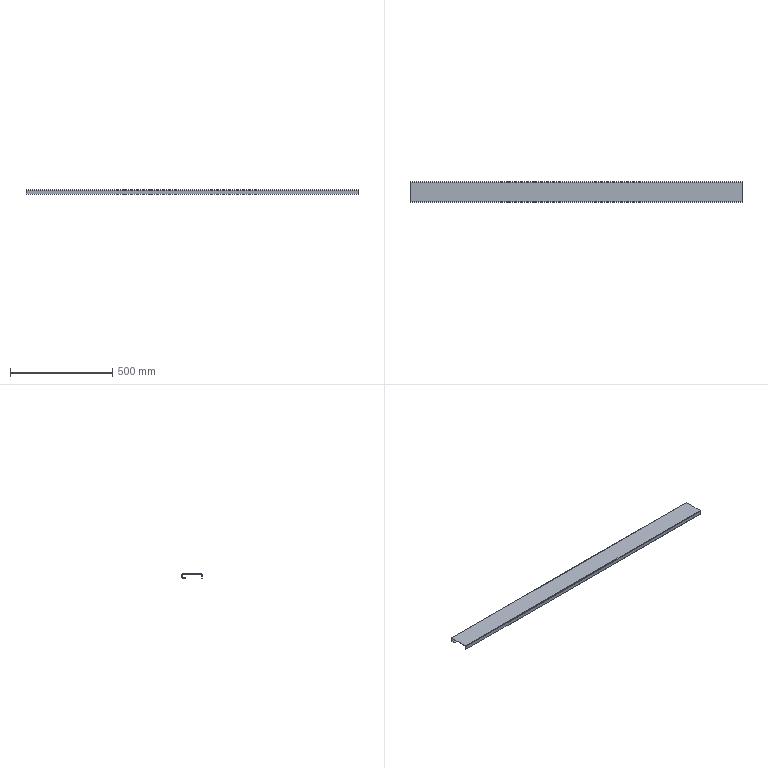Part | STEP file | E3-电柜护栏6踢脚Plate | 1 solid | 18 faces | box 1620 x 100 x 20 mm | volume 372389 mm3 | plane 12 | cylinder 6 | commonest cylinder face diameters 2 x3 5 x3
STEP:
#1=CARTESIAN_POINT('',(0.,0.,0.));
#2=DIRECTION('',(0.,0.,1.));
#3=DIRECTION('',(1.,0.,0.));
#4=AXIS2_PLACEMENT_3D('',#1,#2,#3);
#5=CARTESIAN_POINT('',(-810.,1.5,-2.5));
#6=VERTEX_POINT('',#5);
#7=CARTESIAN_POINT('',(-810.,1.5,-20.));
#8=VERTEX_POINT('',#7);
#9=CARTESIAN_POINT('',(-810.,1.5,-2.5));
#10=DIRECTION('',(0.,0.,-1.));
#11=VECTOR('',#10,1.);
#12=LINE('',#9,#11);
#13=CARTESIAN_POINT('',(810.,1.5,-2.5));
#14=DIRECTION('',(0.,-1.,0.));
#15=DIRECTION('',(0.,0.,1.));
#16=AXIS2_PLACEMENT_3D('',#13,#14,#15);
#17=PLANE('',#16);
#18=CARTESIAN_POINT('',(0.,1620.));
#19=DIRECTION('',(-1.,0.));
#20=VECTOR('',#19,1.);
#21=LINE('',#18,#20);
#22=(GEOMETRIC_REPRESENTATION_CONTEXT(2)PARAMETRIC_REPRESENTATION_CONTEXT()REPRESENTATION_CONTEXT('',''));
#23=DEFINITIONAL_REPRESENTATION('',(#21),#22);
#24=PCURVE('',#17,#23);
#25=CARTESIAN_POINT('',(-810.,2.5,-2.5));
#26=DIRECTION('',(-1.,0.,0.));
#27=DIRECTION('',(0.,0.,-1.));
#28=AXIS2_PLACEMENT_3D('',#25,#26,#27);
#29=PLANE('',#28);
#30=CARTESIAN_POINT('',(0.,1.));
#31=DIRECTION('',(1.,0.));
#32=VECTOR('',#31,1.);
#33=LINE('',#30,#32);
#34=(GEOMETRIC_REPRESENTATION_CONTEXT(2)PARAMETRIC_REPRESENTATION_CONTEXT()REPRESENTATION_CONTEXT('',''));
#35=DEFINITIONAL_REPRESENTATION('',(#33),#34);
#36=PCURVE('',#29,#35);
#37=SURFACE_CURVE('',#12,(#24,#36),.PCURVE_S1.);
#38=EDGE_CURVE('',#6,#8,#37,.T.);
#39=ORIENTED_EDGE('',*,*,#38,.F.);
#40=CARTESIAN_POINT('',(810.,1.5,-2.5));
#41=VERTEX_POINT('',#40);
#42=CARTESIAN_POINT('',(810.,1.5,-2.5));
#43=DIRECTION('',(-1.,0.,0.));
#44=VECTOR('',#43,1.);
#45=LINE('',#42,#44);
#46=CARTESIAN_POINT('',(0.,0.));
#47=DIRECTION('',(0.,1.));
#48=VECTOR('',#47,1.);
#49=LINE('',#46,#48);
#50=(GEOMETRIC_REPRESENTATION_CONTEXT(2)PARAMETRIC_REPRESENTATION_CONTEXT()REPRESENTATION_CONTEXT('',''));
#51=DEFINITIONAL_REPRESENTATION('',(#49),#50);
#52=PCURVE('',#17,#51);
#53=CARTESIAN_POINT('',(810.,2.5,-2.5));
#54=DIRECTION('',(-1.,0.,0.));
#55=DIRECTION('',(0.,0.,-1.));
#56=AXIS2_PLACEMENT_3D('',#53,#54,#55);
#57=CYLINDRICAL_SURFACE('',#56,1.);
#58=CARTESIAN_POINT('',(1.571,0.));
#59=DIRECTION('',(0.,1.));
#60=VECTOR('',#59,1.);
#61=LINE('',#58,#60);
#62=(GEOMETRIC_REPRESENTATION_CONTEXT(2)PARAMETRIC_REPRESENTATION_CONTEXT()REPRESENTATION_CONTEXT('',''));
#63=DEFINITIONAL_REPRESENTATION('',(#61),#62);
#64=PCURVE('',#57,#63);
#65=SURFACE_CURVE('',#45,(#52,#64),.PCURVE_S1.);
#66=EDGE_CURVE('',#41,#6,#65,.T.);
#67=ORIENTED_EDGE('',*,*,#66,.F.);
#68=CARTESIAN_POINT('',(810.,1.5,-20.));
#69=VERTEX_POINT('',#68);
#70=CARTESIAN_POINT('',(810.,1.5,-2.5));
#71=DIRECTION('',(0.,0.,-1.));
#72=VECTOR('',#71,1.);
#73=LINE('',#70,#72);
#74=CARTESIAN_POINT('',(0.,0.));
#75=DIRECTION('',(-1.,0.));
#76=VECTOR('',#75,1.);
#77=LINE('',#74,#76);
#78=(GEOMETRIC_REPRESENTATION_CONTEXT(2)PARAMETRIC_REPRESENTATION_CONTEXT()REPRESENTATION_CONTEXT('',''));
#79=DEFINITIONAL_REPRESENTATION('',(#77),#78);
#80=PCURVE('',#17,#79);
#81=CARTESIAN_POINT('',(810.,2.5,-2.5));
#82=DIRECTION('',(-1.,0.,0.));
#83=DIRECTION('',(0.,0.,-1.));
#84=AXIS2_PLACEMENT_3D('',#81,#82,#83);
#85=PLANE('',#84);
#86=CARTESIAN_POINT('',(0.,1.));
#87=DIRECTION('',(1.,0.));
#88=VECTOR('',#87,1.);
#89=LINE('',#86,#88);
#90=(GEOMETRIC_REPRESENTATION_CONTEXT(2)PARAMETRIC_REPRESENTATION_CONTEXT()REPRESENTATION_CONTEXT('',''));
#91=DEFINITIONAL_REPRESENTATION('',(#89),#90);
#92=PCURVE('',#85,#91);
#93=SURFACE_CURVE('',#73,(#80,#92),.PCURVE_S1.);
#94=EDGE_CURVE('',#41,#69,#93,.T.);
#95=ORIENTED_EDGE('',*,*,#94,.T.);
#96=CARTESIAN_POINT('',(810.,1.5,-20.));
#97=DIRECTION('',(-1.,0.,0.));
#98=VECTOR('',#97,1.);
#99=LINE('',#96,#98);
#100=CARTESIAN_POINT('',(-17.5,0.));
#101=DIRECTION('',(0.,1.));
#102=VECTOR('',#101,1.);
#103=LINE('',#100,#102);
#104=(GEOMETRIC_REPRESENTATION_CONTEXT(2)PARAMETRIC_REPRESENTATION_CONTEXT()REPRESENTATION_CONTEXT('',''));
#105=DEFINITIONAL_REPRESENTATION('',(#103),#104);
#106=PCURVE('',#17,#105);
#107=CARTESIAN_POINT('',(810.,0.,-20.));
#108=DIRECTION('',(0.,0.,-1.));
#109=DIRECTION('',(1.,0.,0.));
#110=AXIS2_PLACEMENT_3D('',#107,#108,#109);
#111=PLANE('',#110);
#112=CARTESIAN_POINT('',(0.,-1.5));
#113=DIRECTION('',(-1.,0.));
#114=VECTOR('',#113,1.);
#115=LINE('',#112,#114);
#116=(GEOMETRIC_REPRESENTATION_CONTEXT(2)PARAMETRIC_REPRESENTATION_CONTEXT()REPRESENTATION_CONTEXT('',''));
#117=DEFINITIONAL_REPRESENTATION('',(#115),#116);
#118=PCURVE('',#111,#117);
#119=SURFACE_CURVE('',#99,(#106,#118),.PCURVE_S1.);
#120=EDGE_CURVE('',#69,#8,#119,.T.);
#121=ORIENTED_EDGE('',*,*,#120,.T.);
#122=EDGE_LOOP('',(#39,#67,#95,#121));
#123=FACE_BOUND('',#122,.T.);
#124=ADVANCED_FACE('',(#123),#17,.F.);
#125=CARTESIAN_POINT('',(-810.,0.,-20.));
#126=VERTEX_POINT('',#125);
#127=CARTESIAN_POINT('',(-810.,0.,-20.));
#128=DIRECTION('',(0.,1.,0.));
#129=VECTOR('',#128,1.);
#130=LINE('',#127,#129);
#131=CARTESIAN_POINT('',(-1620.,0.));
#132=DIRECTION('',(0.,-1.));
#133=VECTOR('',#132,1.);
#134=LINE('',#131,#133);
#135=(GEOMETRIC_REPRESENTATION_CONTEXT(2)PARAMETRIC_REPRESENTATION_CONTEXT()REPRESENTATION_CONTEXT('',''));
#136=DEFINITIONAL_REPRESENTATION('',(#134),#135);
#137=PCURVE('',#111,#136);
#138=CARTESIAN_POINT('',(17.5,2.5));
#139=DIRECTION('',(0.,-1.));
#140=VECTOR('',#139,1.);
#141=LINE('',#138,#140);
#142=(GEOMETRIC_REPRESENTATION_CONTEXT(2)PARAMETRIC_REPRESENTATION_CONTEXT()REPRESENTATION_CONTEXT('',''));
#143=DEFINITIONAL_REPRESENTATION('',(#141),#142);
#144=PCURVE('',#29,#143);
#145=SURFACE_CURVE('',#130,(#137,#144),.PCURVE_S1.);
#146=EDGE_CURVE('',#126,#8,#145,.T.);
#147=ORIENTED_EDGE('',*,*,#146,.T.);
#148=ORIENTED_EDGE('',*,*,#120,.F.);
#149=CARTESIAN_POINT('',(810.,0.,-20.));
#150=VERTEX_POINT('',#149);
#151=CARTESIAN_POINT('',(810.,0.,-20.));
#152=DIRECTION('',(0.,1.,0.));
#153=VECTOR('',#152,1.);
#154=LINE('',#151,#153);
#155=CARTESIAN_POINT('',(0.,0.));
#156=DIRECTION('',(0.,-1.));
#157=VECTOR('',#156,1.);
#158=LINE('',#155,#157);
#159=(GEOMETRIC_REPRESENTATION_CONTEXT(2)PARAMETRIC_REPRESENTATION_CONTEXT()REPRESENTATION_CONTEXT('',''));
#160=DEFINITIONAL_REPRESENTATION('',(#158),#159);
#161=PCURVE('',#111,#160);
#162=CARTESIAN_POINT('',(17.5,2.5));
#163=DIRECTION('',(0.,-1.));
#164=VECTOR('',#163,1.);
#165=LINE('',#162,#164);
#166=(GEOMETRIC_REPRESENTATION_CONTEXT(2)PARAMETRIC_REPRESENTATION_CONTEXT()REPRESENTATION_CONTEXT('',''));
#167=DEFINITIONAL_REPRESENTATION('',(#165),#166);
#168=PCURVE('',#85,#167);
#169=SURFACE_CURVE('',#154,(#161,#168),.PCURVE_S1.);
#170=EDGE_CURVE('',#150,#69,#169,.T.);
#171=ORIENTED_EDGE('',*,*,#170,.F.);
#172=CARTESIAN_POINT('',(810.,0.,-20.));
#173=DIRECTION('',(-1.,0.,0.));
#174=VECTOR('',#173,1.);
#175=LINE('',#172,#174);
#176=CARTESIAN_POINT('',(0.,0.));
#177=DIRECTION('',(-1.,0.));
#178=VECTOR('',#177,1.);
#179=LINE('',#176,#178);
#180=(GEOMETRIC_REPRESENTATION_CONTEXT(2)PARAMETRIC_REPRESENTATION_CONTEXT()REPRESENTATION_CONTEXT('',''));
#181=DEFINITIONAL_REPRESENTATION('',(#179),#180);
#182=PCURVE('',#111,#181);
#183=CARTESIAN_POINT('',(810.,0.,-2.5));
#184=DIRECTION('',(0.,-1.,0.));
#185=DIRECTION('',(0.,0.,1.));
#186=AXIS2_PLACEMENT_3D('',#183,#184,#185);
#187=PLANE('',#186);
#188=CARTESIAN_POINT('',(-17.5,0.));
#189=DIRECTION('',(0.,1.));
#190=VECTOR('',#189,1.);
#191=LINE('',#188,#190);
#192=(GEOMETRIC_REPRESENTATION_CONTEXT(2)PARAMETRIC_REPRESENTATION_CONTEXT()REPRESENTATION_CONTEXT('',''));
#193=DEFINITIONAL_REPRESENTATION('',(#191),#192);
#194=PCURVE('',#187,#193);
#195=SURFACE_CURVE('',#175,(#182,#194),.PCURVE_S1.);
#196=EDGE_CURVE('',#150,#126,#195,.T.);
#197=ORIENTED_EDGE('',*,*,#196,.T.);
#198=EDGE_LOOP('',(#147,#148,#171,#197));
#199=FACE_BOUND('',#198,.T.);
#200=ADVANCED_FACE('',(#199),#111,.T.);
#201=CARTESIAN_POINT('',(-810.,0.,-2.5));
#202=VERTEX_POINT('',#201);
#203=CARTESIAN_POINT('',(-810.,0.,-2.5));
#204=DIRECTION('',(0.,0.,-1.));
#205=VECTOR('',#204,1.);
#206=LINE('',#203,#205);
#207=CARTESIAN_POINT('',(0.,1620.));
#208=DIRECTION('',(-1.,0.));
#209=VECTOR('',#208,1.);
#210=LINE('',#207,#209);
#211=(GEOMETRIC_REPRESENTATION_CONTEXT(2)PARAMETRIC_REPRESENTATION_CONTEXT()REPRESENTATION_CONTEXT('',''));
#212=DEFINITIONAL_REPRESENTATION('',(#210),#211);
#213=PCURVE('',#187,#212);
#214=CARTESIAN_POINT('',(0.,2.5));
#215=DIRECTION('',(1.,0.));
#216=VECTOR('',#215,1.);
#217=LINE('',#214,#216);
#218=(GEOMETRIC_REPRESENTATION_CONTEXT(2)PARAMETRIC_REPRESENTATION_CONTEXT()REPRESENTATION_CONTEXT('',''));
#219=DEFINITIONAL_REPRESENTATION('',(#217),#218);
#220=PCURVE('',#29,#219);
#221=SURFACE_CURVE('',#206,(#213,#220),.PCURVE_S1.);
#222=EDGE_CURVE('',#202,#126,#221,.T.);
#223=ORIENTED_EDGE('',*,*,#222,.T.);
#224=ORIENTED_EDGE('',*,*,#196,.F.);
#225=CARTESIAN_POINT('',(810.,0.,-2.5));
#226=VERTEX_POINT('',#225);
#227=CARTESIAN_POINT('',(810.,0.,-2.5));
#228=DIRECTION('',(0.,0.,-1.));
#229=VECTOR('',#228,1.);
#230=LINE('',#227,#229);
#231=CARTESIAN_POINT('',(0.,0.));
#232=DIRECTION('',(-1.,0.));
#233=VECTOR('',#232,1.);
#234=LINE('',#231,#233);
#235=(GEOMETRIC_REPRESENTATION_CONTEXT(2)PARAMETRIC_REPRESENTATION_CONTEXT()REPRESENTATION_CONTEXT('',''));
#236=DEFINITIONAL_REPRESENTATION('',(#234),#235);
#237=PCURVE('',#187,#236);
#238=CARTESIAN_POINT('',(0.,2.5));
#239=DIRECTION('',(1.,0.));
#240=VECTOR('',#239,1.);
#241=LINE('',#238,#240);
#242=(GEOMETRIC_REPRESENTATION_CONTEXT(2)PARAMETRIC_REPRESENTATION_CONTEXT()REPRESENTATION_CONTEXT('',''));
#243=DEFINITIONAL_REPRESENTATION('',(#241),#242);
#244=PCURVE('',#85,#243);
#245=SURFACE_CURVE('',#230,(#237,#244),.PCURVE_S1.);
#246=EDGE_CURVE('',#226,#150,#245,.T.);
#247=ORIENTED_EDGE('',*,*,#246,.F.);
#248=CARTESIAN_POINT('',(810.,0.,-2.5));
#249=DIRECTION('',(-1.,0.,0.));
#250=VECTOR('',#249,1.);
#251=LINE('',#248,#250);
#252=CARTESIAN_POINT('',(0.,0.));
#253=DIRECTION('',(0.,1.));
#254=VECTOR('',#253,1.);
#255=LINE('',#252,#254);
#256=(GEOMETRIC_REPRESENTATION_CONTEXT(2)PARAMETRIC_REPRESENTATION_CONTEXT()REPRESENTATION_CONTEXT('',''));
#257=DEFINITIONAL_REPRESENTATION('',(#255),#256);
#258=PCURVE('',#187,#257);
#259=CARTESIAN_POINT('',(810.,2.5,-2.5));
#260=DIRECTION('',(-1.,0.,0.));
#261=DIRECTION('',(0.,0.,-1.));
#262=AXIS2_PLACEMENT_3D('',#259,#260,#261);
#263=CYLINDRICAL_SURFACE('',#262,2.5);
#264=CARTESIAN_POINT('',(1.571,0.));
#265=DIRECTION('',(0.,1.));
#266=VECTOR('',#265,1.);
#267=LINE('',#264,#266);
#268=(GEOMETRIC_REPRESENTATION_CONTEXT(2)PARAMETRIC_REPRESENTATION_CONTEXT()REPRESENTATION_CONTEXT('',''));
#269=DEFINITIONAL_REPRESENTATION('',(#267),#268);
#270=PCURVE('',#263,#269);
#271=SURFACE_CURVE('',#251,(#258,#270),.PCURVE_S1.);
#272=EDGE_CURVE('',#226,#202,#271,.T.);
#273=ORIENTED_EDGE('',*,*,#272,.T.);
#274=EDGE_LOOP('',(#223,#224,#247,#273));
#275=FACE_BOUND('',#274,.T.);
#276=ADVANCED_FACE('',(#275),#187,.T.);
#277=CARTESIAN_POINT('',(-810.,2.5,0.));
#278=VERTEX_POINT('',#277);
#279=CARTESIAN_POINT('',(-810.,2.5,-2.5));
#280=DIRECTION('',(1.,0.,0.));
#281=DIRECTION('',(0.,0.,-1.));
#282=AXIS2_PLACEMENT_3D('',#279,#280,#281);
#283=CIRCLE('',#282,2.5);
#284=CARTESIAN_POINT('',(6.283,1620.));
#285=DIRECTION('',(-1.,0.));
#286=VECTOR('',#285,1.);
#287=LINE('',#284,#286);
#288=(GEOMETRIC_REPRESENTATION_CONTEXT(2)PARAMETRIC_REPRESENTATION_CONTEXT()REPRESENTATION_CONTEXT('',''));
#289=DEFINITIONAL_REPRESENTATION('',(#287),#288);
#290=PCURVE('',#263,#289);
#291=CARTESIAN_POINT('',(2.5,0.));
#292=CARTESIAN_POINT('',(2.5,-4.33));
#293=CARTESIAN_POINT('',(-1.25,-2.165));
#294=CARTESIAN_POINT('',(-5.,0.));
#295=CARTESIAN_POINT('',(-1.25,2.165));
#296=CARTESIAN_POINT('',(2.5,4.33));
#297=CARTESIAN_POINT('',(2.5,0.));
#298=(BOUNDED_CURVE()B_SPLINE_CURVE(2,(#291,#292,#293,#294,#295,#296,#297),.UNSPECIFIED.,.T.,.F.)B_SPLINE_CURVE_WITH_KNOTS((1,2,2,2,2,1),(-2.094,0.,2.094,4.189,6.283,8.378),.UNSPECIFIED.)CURVE()GEOMETRIC_REPRESENTATION_ITEM()RATIONAL_B_SPLINE_CURVE((1.,0.5,1.,0.5,1.,0.5,1.))REPRESENTATION_ITEM(''));
#299=(GEOMETRIC_REPRESENTATION_CONTEXT(2)PARAMETRIC_REPRESENTATION_CONTEXT()REPRESENTATION_CONTEXT('',''));
#300=DEFINITIONAL_REPRESENTATION('',(#298),#299);
#301=PCURVE('',#29,#300);
#302=SURFACE_CURVE('',#283,(#290,#301),.PCURVE_S1.);
#303=EDGE_CURVE('',#278,#202,#302,.T.);
#304=ORIENTED_EDGE('',*,*,#303,.T.);
#305=ORIENTED_EDGE('',*,*,#272,.F.);
#306=CARTESIAN_POINT('',(810.,2.5,0.));
#307=VERTEX_POINT('',#306);
#308=CARTESIAN_POINT('',(810.,2.5,-2.5));
#309=DIRECTION('',(1.,0.,0.));
#310=DIRECTION('',(0.,0.,-1.));
#311=AXIS2_PLACEMENT_3D('',#308,#309,#310);
#312=CIRCLE('',#311,2.5);
#313=CARTESIAN_POINT('',(6.283,0.));
#314=DIRECTION('',(-1.,0.));
#315=VECTOR('',#314,1.);
#316=LINE('',#313,#315);
#317=(GEOMETRIC_REPRESENTATION_CONTEXT(2)PARAMETRIC_REPRESENTATION_CONTEXT()REPRESENTATION_CONTEXT('',''));
#318=DEFINITIONAL_REPRESENTATION('',(#316),#317);
#319=PCURVE('',#263,#318);
#320=CARTESIAN_POINT('',(2.5,0.));
#321=CARTESIAN_POINT('',(2.5,-4.33));
#322=CARTESIAN_POINT('',(-1.25,-2.165));
#323=CARTESIAN_POINT('',(-5.,0.));
#324=CARTESIAN_POINT('',(-1.25,2.165));
#325=CARTESIAN_POINT('',(2.5,4.33));
#326=CARTESIAN_POINT('',(2.5,0.));
#327=(BOUNDED_CURVE()B_SPLINE_CURVE(2,(#320,#321,#322,#323,#324,#325,#326),.UNSPECIFIED.,.T.,.F.)B_SPLINE_CURVE_WITH_KNOTS((1,2,2,2,2,1),(-2.094,0.,2.094,4.189,6.283,8.378),.UNSPECIFIED.)CURVE()GEOMETRIC_REPRESENTATION_ITEM()RATIONAL_B_SPLINE_CURVE((1.,0.5,1.,0.5,1.,0.5,1.))REPRESENTATION_ITEM(''));
#328=(GEOMETRIC_REPRESENTATION_CONTEXT(2)PARAMETRIC_REPRESENTATION_CONTEXT()REPRESENTATION_CONTEXT('',''));
#329=DEFINITIONAL_REPRESENTATION('',(#327),#328);
#330=PCURVE('',#85,#329);
#331=SURFACE_CURVE('',#312,(#319,#330),.PCURVE_S1.);
#332=EDGE_CURVE('',#307,#226,#331,.T.);
#333=ORIENTED_EDGE('',*,*,#332,.F.);
#334=CARTESIAN_POINT('',(810.,2.5,0.));
#335=DIRECTION('',(-1.,0.,0.));
#336=VECTOR('',#335,1.);
#337=LINE('',#334,#336);
#338=CARTESIAN_POINT('',(3.142,0.));
#339=DIRECTION('',(0.,1.));
#340=VECTOR('',#339,1.);
#341=LINE('',#338,#340);
#342=(GEOMETRIC_REPRESENTATION_CONTEXT(2)PARAMETRIC_REPRESENTATION_CONTEXT()REPRESENTATION_CONTEXT('',''));
#343=DEFINITIONAL_REPRESENTATION('',(#341),#342);
#344=PCURVE('',#263,#343);
#345=CARTESIAN_POINT('',(810.,2.5,0.));
#346=DIRECTION('',(0.,0.,1.));
#347=DIRECTION('',(-1.,0.,0.));
#348=AXIS2_PLACEMENT_3D('',#345,#346,#347);
#349=PLANE('',#348);
#350=CARTESIAN_POINT('',(0.,0.));
#351=DIRECTION('',(1.,0.));
#352=VECTOR('',#351,1.);
#353=LINE('',#350,#352);
#354=(GEOMETRIC_REPRESENTATION_CONTEXT(2)PARAMETRIC_REPRESENTATION_CONTEXT()REPRESENTATION_CONTEXT('',''));
#355=DEFINITIONAL_REPRESENTATION('',(#353),#354);
#356=PCURVE('',#349,#355);
#357=SURFACE_CURVE('',#337,(#344,#356),.PCURVE_S1.);
#358=EDGE_CURVE('',#307,#278,#357,.T.);
#359=ORIENTED_EDGE('',*,*,#358,.T.);
#360=EDGE_LOOP('',(#304,#305,#333,#359));
#361=FACE_BOUND('',#360,.T.);
#362=ADVANCED_FACE('',(#361),#263,.T.);
#363=CARTESIAN_POINT('',(-810.,97.5,0.));
#364=VERTEX_POINT('',#363);
#365=CARTESIAN_POINT('',(-810.,2.5,0.));
#366=DIRECTION('',(0.,-1.,0.));
#367=VECTOR('',#366,1.);
#368=LINE('',#365,#367);
#369=CARTESIAN_POINT('',(1620.,0.));
#370=DIRECTION('',(0.,1.));
#371=VECTOR('',#370,1.);
#372=LINE('',#369,#371);
#373=(GEOMETRIC_REPRESENTATION_CONTEXT(2)PARAMETRIC_REPRESENTATION_CONTEXT()REPRESENTATION_CONTEXT('',''));
#374=DEFINITIONAL_REPRESENTATION('',(#372),#373);
#375=PCURVE('',#349,#374);
#376=CARTESIAN_POINT('',(-2.5,0.));
#377=DIRECTION('',(0.,1.));
#378=VECTOR('',#377,1.);
#379=LINE('',#376,#378);
#380=(GEOMETRIC_REPRESENTATION_CONTEXT(2)PARAMETRIC_REPRESENTATION_CONTEXT()REPRESENTATION_CONTEXT('',''));
#381=DEFINITIONAL_REPRESENTATION('',(#379),#380);
#382=PCURVE('',#29,#381);
#383=SURFACE_CURVE('',#368,(#375,#382),.PCURVE_S1.);
#384=EDGE_CURVE('',#364,#278,#383,.T.);
#385=ORIENTED_EDGE('',*,*,#384,.T.);
#386=ORIENTED_EDGE('',*,*,#358,.F.);
#387=CARTESIAN_POINT('',(810.,97.5,0.));
#388=VERTEX_POINT('',#387);
#389=CARTESIAN_POINT('',(810.,2.5,0.));
#390=DIRECTION('',(0.,-1.,0.));
#391=VECTOR('',#390,1.);
#392=LINE('',#389,#391);
#393=CARTESIAN_POINT('',(0.,0.));
#394=DIRECTION('',(0.,1.));
#395=VECTOR('',#394,1.);
#396=LINE('',#393,#395);
#397=(GEOMETRIC_REPRESENTATION_CONTEXT(2)PARAMETRIC_REPRESENTATION_CONTEXT()REPRESENTATION_CONTEXT('',''));
#398=DEFINITIONAL_REPRESENTATION('',(#396),#397);
#399=PCURVE('',#349,#398);
#400=CARTESIAN_POINT('',(-2.5,0.));
#401=DIRECTION('',(0.,1.));
#402=VECTOR('',#401,1.);
#403=LINE('',#400,#402);
#404=(GEOMETRIC_REPRESENTATION_CONTEXT(2)PARAMETRIC_REPRESENTATION_CONTEXT()REPRESENTATION_CONTEXT('',''));
#405=DEFINITIONAL_REPRESENTATION('',(#403),#404);
#406=PCURVE('',#85,#405);
#407=SURFACE_CURVE('',#392,(#399,#406),.PCURVE_S1.);
#408=EDGE_CURVE('',#388,#307,#407,.T.);
#409=ORIENTED_EDGE('',*,*,#408,.F.);
#410=CARTESIAN_POINT('',(810.,97.5,0.));
#411=DIRECTION('',(-1.,0.,0.));
#412=VECTOR('',#411,1.);
#413=LINE('',#410,#412);
#414=CARTESIAN_POINT('',(0.,-95.));
#415=DIRECTION('',(1.,0.));
#416=VECTOR('',#415,1.);
#417=LINE('',#414,#416);
#418=(GEOMETRIC_REPRESENTATION_CONTEXT(2)PARAMETRIC_REPRESENTATION_CONTEXT()REPRESENTATION_CONTEXT('',''));
#419=DEFINITIONAL_REPRESENTATION('',(#417),#418);
#420=PCURVE('',#349,#419);
#421=CARTESIAN_POINT('',(810.,97.5,-2.5));
#422=DIRECTION('',(-1.,0.,0.));
#423=DIRECTION('',(0.,0.,-1.));
#424=AXIS2_PLACEMENT_3D('',#421,#422,#423);
#425=CYLINDRICAL_SURFACE('',#424,2.5);
#426=CARTESIAN_POINT('',(3.142,0.));
#427=DIRECTION('',(0.,1.));
#428=VECTOR('',#427,1.);
#429=LINE('',#426,#428);
#430=(GEOMETRIC_REPRESENTATION_CONTEXT(2)PARAMETRIC_REPRESENTATION_CONTEXT()REPRESENTATION_CONTEXT('',''));
#431=DEFINITIONAL_REPRESENTATION('',(#429),#430);
#432=PCURVE('',#425,#431);
#433=SURFACE_CURVE('',#413,(#420,#432),.PCURVE_S1.);
#434=EDGE_CURVE('',#388,#364,#433,.T.);
#435=ORIENTED_EDGE('',*,*,#434,.T.);
#436=EDGE_LOOP('',(#385,#386,#409,#435));
#437=FACE_BOUND('',#436,.T.);
#438=ADVANCED_FACE('',(#437),#349,.T.);
#439=CARTESIAN_POINT('',(-810.,100.,-2.5));
#440=VERTEX_POINT('',#439);
#441=CARTESIAN_POINT('',(-810.,97.5,-2.5));
#442=DIRECTION('',(1.,0.,0.));
#443=DIRECTION('',(0.,0.,1.));
#444=AXIS2_PLACEMENT_3D('',#441,#442,#443);
#445=CIRCLE('',#444,2.5);
#446=CARTESIAN_POINT('',(9.425,1620.));
#447=DIRECTION('',(-1.,0.));
#448=VECTOR('',#447,1.);
#449=LINE('',#446,#448);
#450=(GEOMETRIC_REPRESENTATION_CONTEXT(2)PARAMETRIC_REPRESENTATION_CONTEXT()REPRESENTATION_CONTEXT('',''));
#451=DEFINITIONAL_REPRESENTATION('',(#449),#450);
#452=PCURVE('',#425,#451);
#453=CARTESIAN_POINT('',(-2.5,-95.));
#454=CARTESIAN_POINT('',(-2.5,-90.67));
#455=CARTESIAN_POINT('',(1.25,-92.835));
#456=CARTESIAN_POINT('',(5.,-95.));
#457=CARTESIAN_POINT('',(1.25,-97.165));
#458=CARTESIAN_POINT('',(-2.5,-99.33));
#459=CARTESIAN_POINT('',(-2.5,-95.));
#460=(BOUNDED_CURVE()B_SPLINE_CURVE(2,(#453,#454,#455,#456,#457,#458,#459),.UNSPECIFIED.,.T.,.F.)B_SPLINE_CURVE_WITH_KNOTS((1,2,2,2,2,1),(-2.094,0.,2.094,4.189,6.283,8.378),.UNSPECIFIED.)CURVE()GEOMETRIC_REPRESENTATION_ITEM()RATIONAL_B_SPLINE_CURVE((1.,0.5,1.,0.5,1.,0.5,1.))REPRESENTATION_ITEM(''));
#461=(GEOMETRIC_REPRESENTATION_CONTEXT(2)PARAMETRIC_REPRESENTATION_CONTEXT()REPRESENTATION_CONTEXT('',''));
#462=DEFINITIONAL_REPRESENTATION('',(#460),#461);
#463=PCURVE('',#29,#462);
#464=SURFACE_CURVE('',#445,(#452,#463),.PCURVE_S1.);
#465=EDGE_CURVE('',#440,#364,#464,.T.);
#466=ORIENTED_EDGE('',*,*,#465,.T.);
#467=ORIENTED_EDGE('',*,*,#434,.F.);
#468=CARTESIAN_POINT('',(810.,100.,-2.5));
#469=VERTEX_POINT('',#468);
#470=CARTESIAN_POINT('',(810.,97.5,-2.5));
#471=DIRECTION('',(1.,0.,0.));
#472=DIRECTION('',(0.,0.,1.));
#473=AXIS2_PLACEMENT_3D('',#470,#471,#472);
#474=CIRCLE('',#473,2.5);
#475=CARTESIAN_POINT('',(9.425,0.));
#476=DIRECTION('',(-1.,0.));
#477=VECTOR('',#476,1.);
#478=LINE('',#475,#477);
#479=(GEOMETRIC_REPRESENTATION_CONTEXT(2)PARAMETRIC_REPRESENTATION_CONTEXT()REPRESENTATION_CONTEXT('',''));
#480=DEFINITIONAL_REPRESENTATION('',(#478),#479);
#481=PCURVE('',#425,#480);
#482=CARTESIAN_POINT('',(-2.5,-95.));
#483=CARTESIAN_POINT('',(-2.5,-90.67));
#484=CARTESIAN_POINT('',(1.25,-92.835));
#485=CARTESIAN_POINT('',(5.,-95.));
#486=CARTESIAN_POINT('',(1.25,-97.165));
#487=CARTESIAN_POINT('',(-2.5,-99.33));
#488=CARTESIAN_POINT('',(-2.5,-95.));
#489=(BOUNDED_CURVE()B_SPLINE_CURVE(2,(#482,#483,#484,#485,#486,#487,#488),.UNSPECIFIED.,.T.,.F.)B_SPLINE_CURVE_WITH_KNOTS((1,2,2,2,2,1),(-2.094,0.,2.094,4.189,6.283,8.378),.UNSPECIFIED.)CURVE()GEOMETRIC_REPRESENTATION_ITEM()RATIONAL_B_SPLINE_CURVE((1.,0.5,1.,0.5,1.,0.5,1.))REPRESENTATION_ITEM(''));
#490=(GEOMETRIC_REPRESENTATION_CONTEXT(2)PARAMETRIC_REPRESENTATION_CONTEXT()REPRESENTATION_CONTEXT('',''));
#491=DEFINITIONAL_REPRESENTATION('',(#489),#490);
#492=PCURVE('',#85,#491);
#493=SURFACE_CURVE('',#474,(#481,#492),.PCURVE_S1.);
#494=EDGE_CURVE('',#469,#388,#493,.T.);
#495=ORIENTED_EDGE('',*,*,#494,.F.);
#496=CARTESIAN_POINT('',(810.,100.,-2.5));
#497=DIRECTION('',(-1.,0.,0.));
#498=VECTOR('',#497,1.);
#499=LINE('',#496,#498);
#500=CARTESIAN_POINT('',(4.712,0.));
#501=DIRECTION('',(0.,1.));
#502=VECTOR('',#501,1.);
#503=LINE('',#500,#502);
#504=(GEOMETRIC_REPRESENTATION_CONTEXT(2)PARAMETRIC_REPRESENTATION_CONTEXT()REPRESENTATION_CONTEXT('',''));
#505=DEFINITIONAL_REPRESENTATION('',(#503),#504);
#506=PCURVE('',#425,#505);
#507=CARTESIAN_POINT('',(810.,100.,-2.5));
#508=DIRECTION('',(0.,1.,0.));
#509=DIRECTION('',(0.,0.,-1.));
#510=AXIS2_PLACEMENT_3D('',#507,#508,#509);
#511=PLANE('',#510);
#512=CARTESIAN_POINT('',(0.,0.));
#513=DIRECTION('',(0.,1.));
#514=VECTOR('',#513,1.);
#515=LINE('',#512,#514);
#516=(GEOMETRIC_REPRESENTATION_CONTEXT(2)PARAMETRIC_REPRESENTATION_CONTEXT()REPRESENTATION_CONTEXT('',''));
#517=DEFINITIONAL_REPRESENTATION('',(#515),#516);
#518=PCURVE('',#511,#517);
#519=SURFACE_CURVE('',#499,(#506,#518),.PCURVE_S1.);
#520=EDGE_CURVE('',#469,#440,#519,.T.);
#521=ORIENTED_EDGE('',*,*,#520,.T.);
#522=EDGE_LOOP('',(#466,#467,#495,#521));
#523=FACE_BOUND('',#522,.T.);
#524=ADVANCED_FACE('',(#523),#425,.T.);
#525=CARTESIAN_POINT('',(-810.,100.,-17.5));
#526=VERTEX_POINT('',#525);
#527=CARTESIAN_POINT('',(-810.,100.,-2.5));
#528=DIRECTION('',(0.,0.,1.));
#529=VECTOR('',#528,1.);
#530=LINE('',#527,#529);
#531=CARTESIAN_POINT('',(0.,1620.));
#532=DIRECTION('',(-1.,0.));
#533=VECTOR('',#532,1.);
#534=LINE('',#531,#533);
#535=(GEOMETRIC_REPRESENTATION_CONTEXT(2)PARAMETRIC_REPRESENTATION_CONTEXT()REPRESENTATION_CONTEXT('',''));
#536=DEFINITIONAL_REPRESENTATION('',(#534),#535);
#537=PCURVE('',#511,#536);
#538=CARTESIAN_POINT('',(0.,-97.5));
#539=DIRECTION('',(-1.,0.));
#540=VECTOR('',#539,1.);
#541=LINE('',#538,#540);
#542=(GEOMETRIC_REPRESENTATION_CONTEXT(2)PARAMETRIC_REPRESENTATION_CONTEXT()REPRESENTATION_CONTEXT('',''));
#543=DEFINITIONAL_REPRESENTATION('',(#541),#542);
#544=PCURVE('',#29,#543);
#545=SURFACE_CURVE('',#530,(#537,#544),.PCURVE_S1.);
#546=EDGE_CURVE('',#526,#440,#545,.T.);
#547=ORIENTED_EDGE('',*,*,#546,.T.);
#548=ORIENTED_EDGE('',*,*,#520,.F.);
#549=CARTESIAN_POINT('',(810.,100.,-17.5));
#550=VERTEX_POINT('',#549);
#551=CARTESIAN_POINT('',(810.,100.,-2.5));
#552=DIRECTION('',(0.,0.,1.));
#553=VECTOR('',#552,1.);
#554=LINE('',#551,#553);
#555=CARTESIAN_POINT('',(0.,0.));
#556=DIRECTION('',(-1.,0.));
#557=VECTOR('',#556,1.);
#558=LINE('',#555,#557);
#559=(GEOMETRIC_REPRESENTATION_CONTEXT(2)PARAMETRIC_REPRESENTATION_CONTEXT()REPRESENTATION_CONTEXT('',''));
#560=DEFINITIONAL_REPRESENTATION('',(#558),#559);
#561=PCURVE('',#511,#560);
#562=CARTESIAN_POINT('',(0.,-97.5));
#563=DIRECTION('',(-1.,0.));
#564=VECTOR('',#563,1.);
#565=LINE('',#562,#564);
#566=(GEOMETRIC_REPRESENTATION_CONTEXT(2)PARAMETRIC_REPRESENTATION_CONTEXT()REPRESENTATION_CONTEXT('',''));
#567=DEFINITIONAL_REPRESENTATION('',(#565),#566);
#568=PCURVE('',#85,#567);
#569=SURFACE_CURVE('',#554,(#561,#568),.PCURVE_S1.);
#570=EDGE_CURVE('',#550,#469,#569,.T.);
#571=ORIENTED_EDGE('',*,*,#570,.F.);
#572=CARTESIAN_POINT('',(810.,100.,-17.5));
#573=DIRECTION('',(-1.,0.,0.));
#574=VECTOR('',#573,1.);
#575=LINE('',#572,#574);
#576=CARTESIAN_POINT('',(15.,0.));
#577=DIRECTION('',(0.,1.));
#578=VECTOR('',#577,1.);
#579=LINE('',#576,#578);
#580=(GEOMETRIC_REPRESENTATION_CONTEXT(2)PARAMETRIC_REPRESENTATION_CONTEXT()REPRESENTATION_CONTEXT('',''));
#581=DEFINITIONAL_REPRESENTATION('',(#579),#580);
#582=PCURVE('',#511,#581);
#583=CARTESIAN_POINT('',(810.,97.5,-17.5));
#584=DIRECTION('',(-1.,0.,0.));
#585=DIRECTION('',(0.,0.,-1.));
#586=AXIS2_PLACEMENT_3D('',#583,#584,#585);
#587=CYLINDRICAL_SURFACE('',#586,2.5);
#588=CARTESIAN_POINT('',(4.712,0.));
#589=DIRECTION('',(0.,1.));
#590=VECTOR('',#589,1.);
#591=LINE('',#588,#590);
#592=(GEOMETRIC_REPRESENTATION_CONTEXT(2)PARAMETRIC_REPRESENTATION_CONTEXT()REPRESENTATION_CONTEXT('',''));
#593=DEFINITIONAL_REPRESENTATION('',(#591),#592);
#594=PCURVE('',#587,#593);
#595=SURFACE_CURVE('',#575,(#582,#594),.PCURVE_S1.);
#596=EDGE_CURVE('',#550,#526,#595,.T.);
#597=ORIENTED_EDGE('',*,*,#596,.T.);
#598=EDGE_LOOP('',(#547,#548,#571,#597));
#599=FACE_BOUND('',#598,.T.);
#600=ADVANCED_FACE('',(#599),#511,.T.);
#601=CARTESIAN_POINT('',(-810.,97.5,-20.));
#602=VERTEX_POINT('',#601);
#603=CARTESIAN_POINT('',(-810.,97.5,-17.5));
#604=DIRECTION('',(1.,0.,0.));
#605=DIRECTION('',(0.,0.,1.));
#606=AXIS2_PLACEMENT_3D('',#603,#604,#605);
#607=CIRCLE('',#606,2.5);
#608=CARTESIAN_POINT('',(9.425,1620.));
#609=DIRECTION('',(-1.,0.));
#610=VECTOR('',#609,1.);
#611=LINE('',#608,#610);
#612=(GEOMETRIC_REPRESENTATION_CONTEXT(2)PARAMETRIC_REPRESENTATION_CONTEXT()REPRESENTATION_CONTEXT('',''));
#613=DEFINITIONAL_REPRESENTATION('',(#611),#612);
#614=PCURVE('',#587,#613);
#615=CARTESIAN_POINT('',(12.5,-95.));
#616=CARTESIAN_POINT('',(12.5,-90.67));
#617=CARTESIAN_POINT('',(16.25,-92.835));
#618=CARTESIAN_POINT('',(20.,-95.));
#619=CARTESIAN_POINT('',(16.25,-97.165));
#620=CARTESIAN_POINT('',(12.5,-99.33));
#621=CARTESIAN_POINT('',(12.5,-95.));
#622=(BOUNDED_CURVE()B_SPLINE_CURVE(2,(#615,#616,#617,#618,#619,#620,#621),.UNSPECIFIED.,.T.,.F.)B_SPLINE_CURVE_WITH_KNOTS((1,2,2,2,2,1),(-2.094,0.,2.094,4.189,6.283,8.378),.UNSPECIFIED.)CURVE()GEOMETRIC_REPRESENTATION_ITEM()RATIONAL_B_SPLINE_CURVE((1.,0.5,1.,0.5,1.,0.5,1.))REPRESENTATION_ITEM(''));
#623=(GEOMETRIC_REPRESENTATION_CONTEXT(2)PARAMETRIC_REPRESENTATION_CONTEXT()REPRESENTATION_CONTEXT('',''));
#624=DEFINITIONAL_REPRESENTATION('',(#622),#623);
#625=PCURVE('',#29,#624);
#626=SURFACE_CURVE('',#607,(#614,#625),.PCURVE_S1.);
#627=EDGE_CURVE('',#602,#526,#626,.T.);
#628=ORIENTED_EDGE('',*,*,#627,.T.);
#629=ORIENTED_EDGE('',*,*,#596,.F.);
#630=CARTESIAN_POINT('',(810.,97.5,-20.));
#631=VERTEX_POINT('',#630);
#632=CARTESIAN_POINT('',(810.,97.5,-17.5));
#633=DIRECTION('',(1.,0.,0.));
#634=DIRECTION('',(0.,0.,1.));
#635=AXIS2_PLACEMENT_3D('',#632,#633,#634);
#636=CIRCLE('',#635,2.5);
#637=CARTESIAN_POINT('',(9.425,0.));
#638=DIRECTION('',(-1.,0.));
#639=VECTOR('',#638,1.);
#640=LINE('',#637,#639);
#641=(GEOMETRIC_REPRESENTATION_CONTEXT(2)PARAMETRIC_REPRESENTATION_CONTEXT()REPRESENTATION_CONTEXT('',''));
#642=DEFINITIONAL_REPRESENTATION('',(#640),#641);
#643=PCURVE('',#587,#642);
#644=CARTESIAN_POINT('',(12.5,-95.));
#645=CARTESIAN_POINT('',(12.5,-90.67));
#646=CARTESIAN_POINT('',(16.25,-92.835));
#647=CARTESIAN_POINT('',(20.,-95.));
#648=CARTESIAN_POINT('',(16.25,-97.165));
#649=CARTESIAN_POINT('',(12.5,-99.33));
#650=CARTESIAN_POINT('',(12.5,-95.));
#651=(BOUNDED_CURVE()B_SPLINE_CURVE(2,(#644,#645,#646,#647,#648,#649,#650),.UNSPECIFIED.,.T.,.F.)B_SPLINE_CURVE_WITH_KNOTS((1,2,2,2,2,1),(-2.094,0.,2.094,4.189,6.283,8.378),.UNSPECIFIED.)CURVE()GEOMETRIC_REPRESENTATION_ITEM()RATIONAL_B_SPLINE_CURVE((1.,0.5,1.,0.5,1.,0.5,1.))REPRESENTATION_ITEM(''));
#652=(GEOMETRIC_REPRESENTATION_CONTEXT(2)PARAMETRIC_REPRESENTATION_CONTEXT()REPRESENTATION_CONTEXT('',''));
#653=DEFINITIONAL_REPRESENTATION('',(#651),#652);
#654=PCURVE('',#85,#653);
#655=SURFACE_CURVE('',#636,(#643,#654),.PCURVE_S1.);
#656=EDGE_CURVE('',#631,#550,#655,.T.);
#657=ORIENTED_EDGE('',*,*,#656,.F.);
#658=CARTESIAN_POINT('',(810.,97.5,-20.));
#659=DIRECTION('',(-1.,0.,0.));
#660=VECTOR('',#659,1.);
#661=LINE('',#658,#660);
#662=CARTESIAN_POINT('',(6.283,0.));
#663=DIRECTION('',(0.,1.));
#664=VECTOR('',#663,1.);
#665=LINE('',#662,#664);
#666=(GEOMETRIC_REPRESENTATION_CONTEXT(2)PARAMETRIC_REPRESENTATION_CONTEXT()REPRESENTATION_CONTEXT('',''));
#667=DEFINITIONAL_REPRESENTATION('',(#665),#666);
#668=PCURVE('',#587,#667);
#669=CARTESIAN_POINT('',(810.,97.5,-20.));
#670=DIRECTION('',(0.,0.,-1.));
#671=DIRECTION('',(1.,0.,0.));
#672=AXIS2_PLACEMENT_3D('',#669,#670,#671);
#673=PLANE('',#672);
#674=CARTESIAN_POINT('',(0.,0.));
#675=DIRECTION('',(-1.,0.));
#676=VECTOR('',#675,1.);
#677=LINE('',#674,#676);
#678=(GEOMETRIC_REPRESENTATION_CONTEXT(2)PARAMETRIC_REPRESENTATION_CONTEXT()REPRESENTATION_CONTEXT('',''));
#679=DEFINITIONAL_REPRESENTATION('',(#677),#678);
#680=PCURVE('',#673,#679);
#681=SURFACE_CURVE('',#661,(#668,#680),.PCURVE_S1.);
#682=EDGE_CURVE('',#631,#602,#681,.T.);
#683=ORIENTED_EDGE('',*,*,#682,.T.);
#684=EDGE_LOOP('',(#628,#629,#657,#683));
#685=FACE_BOUND('',#684,.T.);
#686=ADVANCED_FACE('',(#685),#587,.T.);
#687=CARTESIAN_POINT('',(-810.,80.,-20.));
#688=VERTEX_POINT('',#687);
#689=CARTESIAN_POINT('',(-810.,97.5,-20.));
#690=DIRECTION('',(0.,1.,0.));
#691=VECTOR('',#690,1.);
#692=LINE('',#689,#691);
#693=CARTESIAN_POINT('',(-1620.,0.));
#694=DIRECTION('',(0.,-1.));
#695=VECTOR('',#694,1.);
#696=LINE('',#693,#695);
#697=(GEOMETRIC_REPRESENTATION_CONTEXT(2)PARAMETRIC_REPRESENTATION_CONTEXT()REPRESENTATION_CONTEXT('',''));
#698=DEFINITIONAL_REPRESENTATION('',(#696),#697);
#699=PCURVE('',#673,#698);
#700=CARTESIAN_POINT('',(17.5,-95.));
#701=DIRECTION('',(0.,-1.));
#702=VECTOR('',#701,1.);
#703=LINE('',#700,#702);
#704=(GEOMETRIC_REPRESENTATION_CONTEXT(2)PARAMETRIC_REPRESENTATION_CONTEXT()REPRESENTATION_CONTEXT('',''));
#705=DEFINITIONAL_REPRESENTATION('',(#703),#704);
#706=PCURVE('',#29,#705);
#707=SURFACE_CURVE('',#692,(#699,#706),.PCURVE_S1.);
#708=EDGE_CURVE('',#688,#602,#707,.T.);
#709=ORIENTED_EDGE('',*,*,#708,.T.);
#710=ORIENTED_EDGE('',*,*,#682,.F.);
#711=CARTESIAN_POINT('',(810.,80.,-20.));
#712=VERTEX_POINT('',#711);
#713=CARTESIAN_POINT('',(810.,97.5,-20.));
#714=DIRECTION('',(0.,1.,0.));
#715=VECTOR('',#714,1.);
#716=LINE('',#713,#715);
#717=CARTESIAN_POINT('',(0.,0.));
#718=DIRECTION('',(0.,-1.));
#719=VECTOR('',#718,1.);
#720=LINE('',#717,#719);
#721=(GEOMETRIC_REPRESENTATION_CONTEXT(2)PARAMETRIC_REPRESENTATION_CONTEXT()REPRESENTATION_CONTEXT('',''));
#722=DEFINITIONAL_REPRESENTATION('',(#720),#721);
#723=PCURVE('',#673,#722);
#724=CARTESIAN_POINT('',(17.5,-95.));
#725=DIRECTION('',(0.,-1.));
#726=VECTOR('',#725,1.);
#727=LINE('',#724,#726);
#728=(GEOMETRIC_REPRESENTATION_CONTEXT(2)PARAMETRIC_REPRESENTATION_CONTEXT()REPRESENTATION_CONTEXT('',''));
#729=DEFINITIONAL_REPRESENTATION('',(#727),#728);
#730=PCURVE('',#85,#729);
#731=SURFACE_CURVE('',#716,(#723,#730),.PCURVE_S1.);
#732=EDGE_CURVE('',#712,#631,#731,.T.);
#733=ORIENTED_EDGE('',*,*,#732,.F.);
#734=CARTESIAN_POINT('',(810.,80.,-20.));
#735=DIRECTION('',(-1.,0.,0.));
#736=VECTOR('',#735,1.);
#737=LINE('',#734,#736);
#738=CARTESIAN_POINT('',(0.,17.5));
#739=DIRECTION('',(-1.,0.));
#740=VECTOR('',#739,1.);
#741=LINE('',#738,#740);
#742=(GEOMETRIC_REPRESENTATION_CONTEXT(2)PARAMETRIC_REPRESENTATION_CONTEXT()REPRESENTATION_CONTEXT('',''));
#743=DEFINITIONAL_REPRESENTATION('',(#741),#742);
#744=PCURVE('',#673,#743);
#745=CARTESIAN_POINT('',(810.,80.,-18.5));
#746=DIRECTION('',(0.,-1.,0.));
#747=DIRECTION('',(0.,0.,1.));
#748=AXIS2_PLACEMENT_3D('',#745,#746,#747);
#749=PLANE('',#748);
#750=CARTESIAN_POINT('',(-1.5,0.));
#751=DIRECTION('',(0.,1.));
#752=VECTOR('',#751,1.);
#753=LINE('',#750,#752);
#754=(GEOMETRIC_REPRESENTATION_CONTEXT(2)PARAMETRIC_REPRESENTATION_CONTEXT()REPRESENTATION_CONTEXT('',''));
#755=DEFINITIONAL_REPRESENTATION('',(#753),#754);
#756=PCURVE('',#749,#755);
#757=SURFACE_CURVE('',#737,(#744,#756),.PCURVE_S1.);
#758=EDGE_CURVE('',#712,#688,#757,.T.);
#759=ORIENTED_EDGE('',*,*,#758,.T.);
#760=EDGE_LOOP('',(#709,#710,#733,#759));
#761=FACE_BOUND('',#760,.T.);
#762=ADVANCED_FACE('',(#761),#673,.T.);
#763=CARTESIAN_POINT('',(-810.,80.,-18.5));
#764=VERTEX_POINT('',#763);
#765=CARTESIAN_POINT('',(-810.,80.,-18.5));
#766=DIRECTION('',(0.,0.,-1.));
#767=VECTOR('',#766,1.);
#768=LINE('',#765,#767);
#769=CARTESIAN_POINT('',(0.,1620.));
#770=DIRECTION('',(-1.,0.));
#771=VECTOR('',#770,1.);
#772=LINE('',#769,#771);
#773=(GEOMETRIC_REPRESENTATION_CONTEXT(2)PARAMETRIC_REPRESENTATION_CONTEXT()REPRESENTATION_CONTEXT('',''));
#774=DEFINITIONAL_REPRESENTATION('',(#772),#773);
#775=PCURVE('',#749,#774);
#776=CARTESIAN_POINT('',(16.,-77.5));
#777=DIRECTION('',(1.,0.));
#778=VECTOR('',#777,1.);
#779=LINE('',#776,#778);
#780=(GEOMETRIC_REPRESENTATION_CONTEXT(2)PARAMETRIC_REPRESENTATION_CONTEXT()REPRESENTATION_CONTEXT('',''));
#781=DEFINITIONAL_REPRESENTATION('',(#779),#780);
#782=PCURVE('',#29,#781);
#783=SURFACE_CURVE('',#768,(#775,#782),.PCURVE_S1.);
#784=EDGE_CURVE('',#764,#688,#783,.T.);
#785=ORIENTED_EDGE('',*,*,#784,.T.);
#786=ORIENTED_EDGE('',*,*,#758,.F.);
#787=CARTESIAN_POINT('',(810.,80.,-18.5));
#788=VERTEX_POINT('',#787);
#789=CARTESIAN_POINT('',(810.,80.,-18.5));
#790=DIRECTION('',(0.,0.,-1.));
#791=VECTOR('',#790,1.);
#792=LINE('',#789,#791);
#793=CARTESIAN_POINT('',(0.,0.));
#794=DIRECTION('',(-1.,0.));
#795=VECTOR('',#794,1.);
#796=LINE('',#793,#795);
#797=(GEOMETRIC_REPRESENTATION_CONTEXT(2)PARAMETRIC_REPRESENTATION_CONTEXT()REPRESENTATION_CONTEXT('',''));
#798=DEFINITIONAL_REPRESENTATION('',(#796),#797);
#799=PCURVE('',#749,#798);
#800=CARTESIAN_POINT('',(16.,-77.5));
#801=DIRECTION('',(1.,0.));
#802=VECTOR('',#801,1.);
#803=LINE('',#800,#802);
#804=(GEOMETRIC_REPRESENTATION_CONTEXT(2)PARAMETRIC_REPRESENTATION_CONTEXT()REPRESENTATION_CONTEXT('',''));
#805=DEFINITIONAL_REPRESENTATION('',(#803),#804);
#806=PCURVE('',#85,#805);
#807=SURFACE_CURVE('',#792,(#799,#806),.PCURVE_S1.);
#808=EDGE_CURVE('',#788,#712,#807,.T.);
#809=ORIENTED_EDGE('',*,*,#808,.F.);
#810=CARTESIAN_POINT('',(810.,80.,-18.5));
#811=DIRECTION('',(-1.,0.,0.));
#812=VECTOR('',#811,1.);
#813=LINE('',#810,#812);
#814=CARTESIAN_POINT('',(0.,0.));
#815=DIRECTION('',(0.,1.));
#816=VECTOR('',#815,1.);
#817=LINE('',#814,#816);
#818=(GEOMETRIC_REPRESENTATION_CONTEXT(2)PARAMETRIC_REPRESENTATION_CONTEXT()REPRESENTATION_CONTEXT('',''));
#819=DEFINITIONAL_REPRESENTATION('',(#817),#818);
#820=PCURVE('',#749,#819);
#821=CARTESIAN_POINT('',(810.,97.5,-18.5));
#822=DIRECTION('',(0.,0.,-1.));
#823=DIRECTION('',(1.,0.,0.));
#824=AXIS2_PLACEMENT_3D('',#821,#822,#823);
#825=PLANE('',#824);
#826=CARTESIAN_POINT('',(0.,17.5));
#827=DIRECTION('',(-1.,0.));
#828=VECTOR('',#827,1.);
#829=LINE('',#826,#828);
#830=(GEOMETRIC_REPRESENTATION_CONTEXT(2)PARAMETRIC_REPRESENTATION_CONTEXT()REPRESENTATION_CONTEXT('',''));
#831=DEFINITIONAL_REPRESENTATION('',(#829),#830);
#832=PCURVE('',#825,#831);
#833=SURFACE_CURVE('',#813,(#820,#832),.PCURVE_S1.);
#834=EDGE_CURVE('',#788,#764,#833,.T.);
#835=ORIENTED_EDGE('',*,*,#834,.T.);
#836=EDGE_LOOP('',(#785,#786,#809,#835));
#837=FACE_BOUND('',#836,.T.);
#838=ADVANCED_FACE('',(#837),#749,.T.);
#839=CARTESIAN_POINT('',(-810.,97.5,-18.5));
#840=VERTEX_POINT('',#839);
#841=CARTESIAN_POINT('',(-810.,97.5,-18.5));
#842=DIRECTION('',(0.,1.,0.));
#843=VECTOR('',#842,1.);
#844=LINE('',#841,#843);
#845=CARTESIAN_POINT('',(-1620.,0.));
#846=DIRECTION('',(0.,-1.));
#847=VECTOR('',#846,1.);
#848=LINE('',#845,#847);
#849=(GEOMETRIC_REPRESENTATION_CONTEXT(2)PARAMETRIC_REPRESENTATION_CONTEXT()REPRESENTATION_CONTEXT('',''));
#850=DEFINITIONAL_REPRESENTATION('',(#848),#849);
#851=PCURVE('',#825,#850);
#852=CARTESIAN_POINT('',(16.,-95.));
#853=DIRECTION('',(0.,-1.));
#854=VECTOR('',#853,1.);
#855=LINE('',#852,#854);
#856=(GEOMETRIC_REPRESENTATION_CONTEXT(2)PARAMETRIC_REPRESENTATION_CONTEXT()REPRESENTATION_CONTEXT('',''));
#857=DEFINITIONAL_REPRESENTATION('',(#855),#856);
#858=PCURVE('',#29,#857);
#859=SURFACE_CURVE('',#844,(#851,#858),.PCURVE_S1.);
#860=EDGE_CURVE('',#764,#840,#859,.T.);
#861=ORIENTED_EDGE('',*,*,#860,.F.);
#862=ORIENTED_EDGE('',*,*,#834,.F.);
#863=CARTESIAN_POINT('',(810.,97.5,-18.5));
#864=VERTEX_POINT('',#863);
#865=CARTESIAN_POINT('',(810.,97.5,-18.5));
#866=DIRECTION('',(0.,1.,0.));
#867=VECTOR('',#866,1.);
#868=LINE('',#865,#867);
#869=CARTESIAN_POINT('',(0.,0.));
#870=DIRECTION('',(0.,-1.));
#871=VECTOR('',#870,1.);
#872=LINE('',#869,#871);
#873=(GEOMETRIC_REPRESENTATION_CONTEXT(2)PARAMETRIC_REPRESENTATION_CONTEXT()REPRESENTATION_CONTEXT('',''));
#874=DEFINITIONAL_REPRESENTATION('',(#872),#873);
#875=PCURVE('',#825,#874);
#876=CARTESIAN_POINT('',(16.,-95.));
#877=DIRECTION('',(0.,-1.));
#878=VECTOR('',#877,1.);
#879=LINE('',#876,#878);
#880=(GEOMETRIC_REPRESENTATION_CONTEXT(2)PARAMETRIC_REPRESENTATION_CONTEXT()REPRESENTATION_CONTEXT('',''));
#881=DEFINITIONAL_REPRESENTATION('',(#879),#880);
#882=PCURVE('',#85,#881);
#883=SURFACE_CURVE('',#868,(#875,#882),.PCURVE_S1.);
#884=EDGE_CURVE('',#788,#864,#883,.T.);
#885=ORIENTED_EDGE('',*,*,#884,.T.);
#886=CARTESIAN_POINT('',(810.,97.5,-18.5));
#887=DIRECTION('',(-1.,0.,0.));
#888=VECTOR('',#887,1.);
#889=LINE('',#886,#888);
#890=CARTESIAN_POINT('',(0.,0.));
#891=DIRECTION('',(-1.,0.));
#892=VECTOR('',#891,1.);
#893=LINE('',#890,#892);
#894=(GEOMETRIC_REPRESENTATION_CONTEXT(2)PARAMETRIC_REPRESENTATION_CONTEXT()REPRESENTATION_CONTEXT('',''));
#895=DEFINITIONAL_REPRESENTATION('',(#893),#894);
#896=PCURVE('',#825,#895);
#897=CARTESIAN_POINT('',(810.,97.5,-17.5));
#898=DIRECTION('',(-1.,0.,0.));
#899=DIRECTION('',(0.,0.,-1.));
#900=AXIS2_PLACEMENT_3D('',#897,#898,#899);
#901=CYLINDRICAL_SURFACE('',#900,1.);
#902=CARTESIAN_POINT('',(6.283,0.));
#903=DIRECTION('',(0.,1.));
#904=VECTOR('',#903,1.);
#905=LINE('',#902,#904);
#906=(GEOMETRIC_REPRESENTATION_CONTEXT(2)PARAMETRIC_REPRESENTATION_CONTEXT()REPRESENTATION_CONTEXT('',''));
#907=DEFINITIONAL_REPRESENTATION('',(#905),#906);
#908=PCURVE('',#901,#907);
#909=SURFACE_CURVE('',#889,(#896,#908),.PCURVE_S1.);
#910=EDGE_CURVE('',#864,#840,#909,.T.);
#911=ORIENTED_EDGE('',*,*,#910,.T.);
#912=EDGE_LOOP('',(#861,#862,#885,#911));
#913=FACE_BOUND('',#912,.T.);
#914=ADVANCED_FACE('',(#913),#825,.F.);
#915=CARTESIAN_POINT('',(810.,98.5,-17.5));
#916=VERTEX_POINT('',#915);
#917=CARTESIAN_POINT('',(-810.,98.5,-17.5));
#918=VERTEX_POINT('',#917);
#919=CARTESIAN_POINT('',(810.,98.5,-17.5));
#920=DIRECTION('',(-1.,0.,0.));
#921=VECTOR('',#920,1.);
#922=LINE('',#919,#921);
#923=CARTESIAN_POINT('',(4.712,0.));
#924=DIRECTION('',(0.,1.));
#925=VECTOR('',#924,1.);
#926=LINE('',#923,#925);
#927=(GEOMETRIC_REPRESENTATION_CONTEXT(2)PARAMETRIC_REPRESENTATION_CONTEXT()REPRESENTATION_CONTEXT('',''));
#928=DEFINITIONAL_REPRESENTATION('',(#926),#927);
#929=PCURVE('',#901,#928);
#930=CARTESIAN_POINT('',(810.,98.5,-2.5));
#931=DIRECTION('',(0.,1.,0.));
#932=DIRECTION('',(0.,0.,-1.));
#933=AXIS2_PLACEMENT_3D('',#930,#931,#932);
#934=PLANE('',#933);
#935=CARTESIAN_POINT('',(15.,0.));
#936=DIRECTION('',(0.,1.));
#937=VECTOR('',#936,1.);
#938=LINE('',#935,#937);
#939=(GEOMETRIC_REPRESENTATION_CONTEXT(2)PARAMETRIC_REPRESENTATION_CONTEXT()REPRESENTATION_CONTEXT('',''));
#940=DEFINITIONAL_REPRESENTATION('',(#938),#939);
#941=PCURVE('',#934,#940);
#942=SURFACE_CURVE('',#922,(#929,#941),.PCURVE_S1.);
#943=EDGE_CURVE('',#916,#918,#942,.T.);
#944=ORIENTED_EDGE('',*,*,#943,.F.);
#945=CARTESIAN_POINT('',(810.,97.5,-17.5));
#946=DIRECTION('',(1.,0.,0.));
#947=DIRECTION('',(0.,0.,1.));
#948=AXIS2_PLACEMENT_3D('',#945,#946,#947);
#949=CIRCLE('',#948,1.);
#950=CARTESIAN_POINT('',(9.425,0.));
#951=DIRECTION('',(-1.,0.));
#952=VECTOR('',#951,1.);
#953=LINE('',#950,#952);
#954=(GEOMETRIC_REPRESENTATION_CONTEXT(2)PARAMETRIC_REPRESENTATION_CONTEXT()REPRESENTATION_CONTEXT('',''));
#955=DEFINITIONAL_REPRESENTATION('',(#953),#954);
#956=PCURVE('',#901,#955);
#957=CARTESIAN_POINT('',(14.,-95.));
#958=CARTESIAN_POINT('',(14.,-93.268));
#959=CARTESIAN_POINT('',(15.5,-94.134));
#960=CARTESIAN_POINT('',(17.,-95.));
#961=CARTESIAN_POINT('',(15.5,-95.866));
#962=CARTESIAN_POINT('',(14.,-96.732));
#963=CARTESIAN_POINT('',(14.,-95.));
#964=(BOUNDED_CURVE()B_SPLINE_CURVE(2,(#957,#958,#959,#960,#961,#962,#963),.UNSPECIFIED.,.T.,.F.)B_SPLINE_CURVE_WITH_KNOTS((1,2,2,2,2,1),(-2.094,0.,2.094,4.189,6.283,8.378),.UNSPECIFIED.)CURVE()GEOMETRIC_REPRESENTATION_ITEM()RATIONAL_B_SPLINE_CURVE((1.,0.5,1.,0.5,1.,0.5,1.))REPRESENTATION_ITEM(''));
#965=(GEOMETRIC_REPRESENTATION_CONTEXT(2)PARAMETRIC_REPRESENTATION_CONTEXT()REPRESENTATION_CONTEXT('',''));
#966=DEFINITIONAL_REPRESENTATION('',(#964),#965);
#967=PCURVE('',#85,#966);
#968=SURFACE_CURVE('',#949,(#956,#967),.PCURVE_S1.);
#969=EDGE_CURVE('',#864,#916,#968,.T.);
#970=ORIENTED_EDGE('',*,*,#969,.F.);
#971=ORIENTED_EDGE('',*,*,#910,.T.);
#972=CARTESIAN_POINT('',(-810.,97.5,-17.5));
#973=DIRECTION('',(1.,0.,0.));
#974=DIRECTION('',(0.,0.,1.));
#975=AXIS2_PLACEMENT_3D('',#972,#973,#974);
#976=CIRCLE('',#975,1.);
#977=CARTESIAN_POINT('',(9.425,1620.));
#978=DIRECTION('',(-1.,0.));
#979=VECTOR('',#978,1.);
#980=LINE('',#977,#979);
#981=(GEOMETRIC_REPRESENTATION_CONTEXT(2)PARAMETRIC_REPRESENTATION_CONTEXT()REPRESENTATION_CONTEXT('',''));
#982=DEFINITIONAL_REPRESENTATION('',(#980),#981);
#983=PCURVE('',#901,#982);
#984=CARTESIAN_POINT('',(14.,-95.));
#985=CARTESIAN_POINT('',(14.,-93.268));
#986=CARTESIAN_POINT('',(15.5,-94.134));
#987=CARTESIAN_POINT('',(17.,-95.));
#988=CARTESIAN_POINT('',(15.5,-95.866));
#989=CARTESIAN_POINT('',(14.,-96.732));
#990=CARTESIAN_POINT('',(14.,-95.));
#991=(BOUNDED_CURVE()B_SPLINE_CURVE(2,(#984,#985,#986,#987,#988,#989,#990),.UNSPECIFIED.,.T.,.F.)B_SPLINE_CURVE_WITH_KNOTS((1,2,2,2,2,1),(-2.094,0.,2.094,4.189,6.283,8.378),.UNSPECIFIED.)CURVE()GEOMETRIC_REPRESENTATION_ITEM()RATIONAL_B_SPLINE_CURVE((1.,0.5,1.,0.5,1.,0.5,1.))REPRESENTATION_ITEM(''));
#992=(GEOMETRIC_REPRESENTATION_CONTEXT(2)PARAMETRIC_REPRESENTATION_CONTEXT()REPRESENTATION_CONTEXT('',''));
#993=DEFINITIONAL_REPRESENTATION('',(#991),#992);
#994=PCURVE('',#29,#993);
#995=SURFACE_CURVE('',#976,(#983,#994),.PCURVE_S1.);
#996=EDGE_CURVE('',#840,#918,#995,.T.);
#997=ORIENTED_EDGE('',*,*,#996,.T.);
#998=EDGE_LOOP('',(#944,#970,#971,#997));
#999=FACE_BOUND('',#998,.F.);
#1000=ADVANCED_FACE('',(#999),#901,.F.);
#1001=CARTESIAN_POINT('',(-810.,98.5,-2.5));
#1002=VERTEX_POINT('',#1001);
#1003=CARTESIAN_POINT('',(-810.,98.5,-2.5));
#1004=DIRECTION('',(0.,0.,1.));
#1005=VECTOR('',#1004,1.);
#1006=LINE('',#1003,#1005);
#1007=CARTESIAN_POINT('',(0.,1620.));
#1008=DIRECTION('',(-1.,0.));
#1009=VECTOR('',#1008,1.);
#1010=LINE('',#1007,#1009);
#1011=(GEOMETRIC_REPRESENTATION_CONTEXT(2)PARAMETRIC_REPRESENTATION_CONTEXT()REPRESENTATION_CONTEXT('',''));
#1012=DEFINITIONAL_REPRESENTATION('',(#1010),#1011);
#1013=PCURVE('',#934,#1012);
#1014=CARTESIAN_POINT('',(0.,-96.));
#1015=DIRECTION('',(-1.,0.));
#1016=VECTOR('',#1015,1.);
#1017=LINE('',#1014,#1016);
#1018=(GEOMETRIC_REPRESENTATION_CONTEXT(2)PARAMETRIC_REPRESENTATION_CONTEXT()REPRESENTATION_CONTEXT('',''));
#1019=DEFINITIONAL_REPRESENTATION('',(#1017),#1018);
#1020=PCURVE('',#29,#1019);
#1021=SURFACE_CURVE('',#1006,(#1013,#1020),.PCURVE_S1.);
#1022=EDGE_CURVE('',#918,#1002,#1021,.T.);
#1023=ORIENTED_EDGE('',*,*,#1022,.F.);
#1024=ORIENTED_EDGE('',*,*,#943,.F.);
#1025=CARTESIAN_POINT('',(810.,98.5,-2.5));
#1026=VERTEX_POINT('',#1025);
#1027=CARTESIAN_POINT('',(810.,98.5,-2.5));
#1028=DIRECTION('',(0.,0.,1.));
#1029=VECTOR('',#1028,1.);
#1030=LINE('',#1027,#1029);
#1031=CARTESIAN_POINT('',(0.,0.));
#1032=DIRECTION('',(-1.,0.));
#1033=VECTOR('',#1032,1.);
#1034=LINE('',#1031,#1033);
#1035=(GEOMETRIC_REPRESENTATION_CONTEXT(2)PARAMETRIC_REPRESENTATION_CONTEXT()REPRESENTATION_CONTEXT('',''));
#1036=DEFINITIONAL_REPRESENTATION('',(#1034),#1035);
#1037=PCURVE('',#934,#1036);
#1038=CARTESIAN_POINT('',(0.,-96.));
#1039=DIRECTION('',(-1.,0.));
#1040=VECTOR('',#1039,1.);
#1041=LINE('',#1038,#1040);
#1042=(GEOMETRIC_REPRESENTATION_CONTEXT(2)PARAMETRIC_REPRESENTATION_CONTEXT()REPRESENTATION_CONTEXT('',''));
#1043=DEFINITIONAL_REPRESENTATION('',(#1041),#1042);
#1044=PCURVE('',#85,#1043);
#1045=SURFACE_CURVE('',#1030,(#1037,#1044),.PCURVE_S1.);
#1046=EDGE_CURVE('',#916,#1026,#1045,.T.);
#1047=ORIENTED_EDGE('',*,*,#1046,.T.);
#1048=CARTESIAN_POINT('',(810.,98.5,-2.5));
#1049=DIRECTION('',(-1.,0.,0.));
#1050=VECTOR('',#1049,1.);
#1051=LINE('',#1048,#1050);
#1052=CARTESIAN_POINT('',(0.,0.));
#1053=DIRECTION('',(0.,1.));
#1054=VECTOR('',#1053,1.);
#1055=LINE('',#1052,#1054);
#1056=(GEOMETRIC_REPRESENTATION_CONTEXT(2)PARAMETRIC_REPRESENTATION_CONTEXT()REPRESENTATION_CONTEXT('',''));
#1057=DEFINITIONAL_REPRESENTATION('',(#1055),#1056);
#1058=PCURVE('',#934,#1057);
#1059=CARTESIAN_POINT('',(810.,97.5,-2.5));
#1060=DIRECTION('',(-1.,0.,0.));
#1061=DIRECTION('',(0.,0.,-1.));
#1062=AXIS2_PLACEMENT_3D('',#1059,#1060,#1061);
#1063=CYLINDRICAL_SURFACE('',#1062,1.);
#1064=CARTESIAN_POINT('',(4.712,0.));
#1065=DIRECTION('',(0.,1.));
#1066=VECTOR('',#1065,1.);
#1067=LINE('',#1064,#1066);
#1068=(GEOMETRIC_REPRESENTATION_CONTEXT(2)PARAMETRIC_REPRESENTATION_CONTEXT()REPRESENTATION_CONTEXT('',''));
#1069=DEFINITIONAL_REPRESENTATION('',(#1067),#1068);
#1070=PCURVE('',#1063,#1069);
#1071=SURFACE_CURVE('',#1051,(#1058,#1070),.PCURVE_S1.);
#1072=EDGE_CURVE('',#1026,#1002,#1071,.T.);
#1073=ORIENTED_EDGE('',*,*,#1072,.T.);
#1074=EDGE_LOOP('',(#1023,#1024,#1047,#1073));
#1075=FACE_BOUND('',#1074,.T.);
#1076=ADVANCED_FACE('',(#1075),#934,.F.);
#1077=CARTESIAN_POINT('',(810.,97.5,-1.5));
#1078=VERTEX_POINT('',#1077);
#1079=CARTESIAN_POINT('',(-810.,97.5,-1.5));
#1080=VERTEX_POINT('',#1079);
#1081=CARTESIAN_POINT('',(810.,97.5,-1.5));
#1082=DIRECTION('',(-1.,0.,0.));
#1083=VECTOR('',#1082,1.);
#1084=LINE('',#1081,#1083);
#1085=CARTESIAN_POINT('',(3.142,0.));
#1086=DIRECTION('',(0.,1.));
#1087=VECTOR('',#1086,1.);
#1088=LINE('',#1085,#1087);
#1089=(GEOMETRIC_REPRESENTATION_CONTEXT(2)PARAMETRIC_REPRESENTATION_CONTEXT()REPRESENTATION_CONTEXT('',''));
#1090=DEFINITIONAL_REPRESENTATION('',(#1088),#1089);
#1091=PCURVE('',#1063,#1090);
#1092=CARTESIAN_POINT('',(810.,2.5,-1.5));
#1093=DIRECTION('',(0.,0.,1.));
#1094=DIRECTION('',(-1.,0.,0.));
#1095=AXIS2_PLACEMENT_3D('',#1092,#1093,#1094);
#1096=PLANE('',#1095);
#1097=CARTESIAN_POINT('',(0.,-95.));
#1098=DIRECTION('',(1.,0.));
#1099=VECTOR('',#1098,1.);
#1100=LINE('',#1097,#1099);
#1101=(GEOMETRIC_REPRESENTATION_CONTEXT(2)PARAMETRIC_REPRESENTATION_CONTEXT()REPRESENTATION_CONTEXT('',''));
#1102=DEFINITIONAL_REPRESENTATION('',(#1100),#1101);
#1103=PCURVE('',#1096,#1102);
#1104=SURFACE_CURVE('',#1084,(#1091,#1103),.PCURVE_S1.);
#1105=EDGE_CURVE('',#1078,#1080,#1104,.T.);
#1106=ORIENTED_EDGE('',*,*,#1105,.F.);
#1107=CARTESIAN_POINT('',(810.,97.5,-2.5));
#1108=DIRECTION('',(1.,0.,0.));
#1109=DIRECTION('',(0.,0.,1.));
#1110=AXIS2_PLACEMENT_3D('',#1107,#1108,#1109);
#1111=CIRCLE('',#1110,1.);
#1112=CARTESIAN_POINT('',(9.425,0.));
#1113=DIRECTION('',(-1.,0.));
#1114=VECTOR('',#1113,1.);
#1115=LINE('',#1112,#1114);
#1116=(GEOMETRIC_REPRESENTATION_CONTEXT(2)PARAMETRIC_REPRESENTATION_CONTEXT()REPRESENTATION_CONTEXT('',''));
#1117=DEFINITIONAL_REPRESENTATION('',(#1115),#1116);
#1118=PCURVE('',#1063,#1117);
#1119=CARTESIAN_POINT('',(-1.,-95.));
#1120=CARTESIAN_POINT('',(-1.,-93.268));
#1121=CARTESIAN_POINT('',(0.5,-94.134));
#1122=CARTESIAN_POINT('',(2.,-95.));
#1123=CARTESIAN_POINT('',(0.5,-95.866));
#1124=CARTESIAN_POINT('',(-1.,-96.732));
#1125=CARTESIAN_POINT('',(-1.,-95.));
#1126=(BOUNDED_CURVE()B_SPLINE_CURVE(2,(#1119,#1120,#1121,#1122,#1123,#1124,#1125),.UNSPECIFIED.,.T.,.F.)B_SPLINE_CURVE_WITH_KNOTS((1,2,2,2,2,1),(-2.094,0.,2.094,4.189,6.283,8.378),.UNSPECIFIED.)CURVE()GEOMETRIC_REPRESENTATION_ITEM()RATIONAL_B_SPLINE_CURVE((1.,0.5,1.,0.5,1.,0.5,1.))REPRESENTATION_ITEM(''));
#1127=(GEOMETRIC_REPRESENTATION_CONTEXT(2)PARAMETRIC_REPRESENTATION_CONTEXT()REPRESENTATION_CONTEXT('',''));
#1128=DEFINITIONAL_REPRESENTATION('',(#1126),#1127);
#1129=PCURVE('',#85,#1128);
#1130=SURFACE_CURVE('',#1111,(#1118,#1129),.PCURVE_S1.);
#1131=EDGE_CURVE('',#1026,#1078,#1130,.T.);
#1132=ORIENTED_EDGE('',*,*,#1131,.F.);
#1133=ORIENTED_EDGE('',*,*,#1072,.T.);
#1134=CARTESIAN_POINT('',(-810.,97.5,-2.5));
#1135=DIRECTION('',(1.,0.,0.));
#1136=DIRECTION('',(0.,0.,1.));
#1137=AXIS2_PLACEMENT_3D('',#1134,#1135,#1136);
#1138=CIRCLE('',#1137,1.);
#1139=CARTESIAN_POINT('',(9.425,1620.));
#1140=DIRECTION('',(-1.,0.));
#1141=VECTOR('',#1140,1.);
#1142=LINE('',#1139,#1141);
#1143=(GEOMETRIC_REPRESENTATION_CONTEXT(2)PARAMETRIC_REPRESENTATION_CONTEXT()REPRESENTATION_CONTEXT('',''));
#1144=DEFINITIONAL_REPRESENTATION('',(#1142),#1143);
#1145=PCURVE('',#1063,#1144);
#1146=CARTESIAN_POINT('',(-1.,-95.));
#1147=CARTESIAN_POINT('',(-1.,-93.268));
#1148=CARTESIAN_POINT('',(0.5,-94.134));
#1149=CARTESIAN_POINT('',(2.,-95.));
#1150=CARTESIAN_POINT('',(0.5,-95.866));
#1151=CARTESIAN_POINT('',(-1.,-96.732));
#1152=CARTESIAN_POINT('',(-1.,-95.));
#1153=(BOUNDED_CURVE()B_SPLINE_CURVE(2,(#1146,#1147,#1148,#1149,#1150,#1151,#1152),.UNSPECIFIED.,.T.,.F.)B_SPLINE_CURVE_WITH_KNOTS((1,2,2,2,2,1),(-2.094,0.,2.094,4.189,6.283,8.378),.UNSPECIFIED.)CURVE()GEOMETRIC_REPRESENTATION_ITEM()RATIONAL_B_SPLINE_CURVE((1.,0.5,1.,0.5,1.,0.5,1.))REPRESENTATION_ITEM(''));
#1154=(GEOMETRIC_REPRESENTATION_CONTEXT(2)PARAMETRIC_REPRESENTATION_CONTEXT()REPRESENTATION_CONTEXT('',''));
#1155=DEFINITIONAL_REPRESENTATION('',(#1153),#1154);
#1156=PCURVE('',#29,#1155);
#1157=SURFACE_CURVE('',#1138,(#1145,#1156),.PCURVE_S1.);
#1158=EDGE_CURVE('',#1002,#1080,#1157,.T.);
#1159=ORIENTED_EDGE('',*,*,#1158,.T.);
#1160=EDGE_LOOP('',(#1106,#1132,#1133,#1159));
#1161=FACE_BOUND('',#1160,.F.);
#1162=ADVANCED_FACE('',(#1161),#1063,.F.);
#1163=CARTESIAN_POINT('',(-810.,2.5,-1.5));
#1164=VERTEX_POINT('',#1163);
#1165=CARTESIAN_POINT('',(-810.,2.5,-1.5));
#1166=DIRECTION('',(0.,-1.,0.));
#1167=VECTOR('',#1166,1.);
#1168=LINE('',#1165,#1167);
#1169=CARTESIAN_POINT('',(1620.,0.));
#1170=DIRECTION('',(0.,1.));
#1171=VECTOR('',#1170,1.);
#1172=LINE('',#1169,#1171);
#1173=(GEOMETRIC_REPRESENTATION_CONTEXT(2)PARAMETRIC_REPRESENTATION_CONTEXT()REPRESENTATION_CONTEXT('',''));
#1174=DEFINITIONAL_REPRESENTATION('',(#1172),#1173);
#1175=PCURVE('',#1096,#1174);
#1176=CARTESIAN_POINT('',(-1.,0.));
#1177=DIRECTION('',(0.,1.));
#1178=VECTOR('',#1177,1.);
#1179=LINE('',#1176,#1178);
#1180=(GEOMETRIC_REPRESENTATION_CONTEXT(2)PARAMETRIC_REPRESENTATION_CONTEXT()REPRESENTATION_CONTEXT('',''));
#1181=DEFINITIONAL_REPRESENTATION('',(#1179),#1180);
#1182=PCURVE('',#29,#1181);
#1183=SURFACE_CURVE('',#1168,(#1175,#1182),.PCURVE_S1.);
#1184=EDGE_CURVE('',#1080,#1164,#1183,.T.);
#1185=ORIENTED_EDGE('',*,*,#1184,.F.);
#1186=ORIENTED_EDGE('',*,*,#1105,.F.);
#1187=CARTESIAN_POINT('',(810.,2.5,-1.5));
#1188=VERTEX_POINT('',#1187);
#1189=CARTESIAN_POINT('',(810.,2.5,-1.5));
#1190=DIRECTION('',(0.,-1.,0.));
#1191=VECTOR('',#1190,1.);
#1192=LINE('',#1189,#1191);
#1193=CARTESIAN_POINT('',(0.,0.));
#1194=DIRECTION('',(0.,1.));
#1195=VECTOR('',#1194,1.);
#1196=LINE('',#1193,#1195);
#1197=(GEOMETRIC_REPRESENTATION_CONTEXT(2)PARAMETRIC_REPRESENTATION_CONTEXT()REPRESENTATION_CONTEXT('',''));
#1198=DEFINITIONAL_REPRESENTATION('',(#1196),#1197);
#1199=PCURVE('',#1096,#1198);
#1200=CARTESIAN_POINT('',(-1.,0.));
#1201=DIRECTION('',(0.,1.));
#1202=VECTOR('',#1201,1.);
#1203=LINE('',#1200,#1202);
#1204=(GEOMETRIC_REPRESENTATION_CONTEXT(2)PARAMETRIC_REPRESENTATION_CONTEXT()REPRESENTATION_CONTEXT('',''));
#1205=DEFINITIONAL_REPRESENTATION('',(#1203),#1204);
#1206=PCURVE('',#85,#1205);
#1207=SURFACE_CURVE('',#1192,(#1199,#1206),.PCURVE_S1.);
#1208=EDGE_CURVE('',#1078,#1188,#1207,.T.);
#1209=ORIENTED_EDGE('',*,*,#1208,.T.);
#1210=CARTESIAN_POINT('',(810.,2.5,-1.5));
#1211=DIRECTION('',(-1.,0.,0.));
#1212=VECTOR('',#1211,1.);
#1213=LINE('',#1210,#1212);
#1214=CARTESIAN_POINT('',(0.,0.));
#1215=DIRECTION('',(1.,0.));
#1216=VECTOR('',#1215,1.);
#1217=LINE('',#1214,#1216);
#1218=(GEOMETRIC_REPRESENTATION_CONTEXT(2)PARAMETRIC_REPRESENTATION_CONTEXT()REPRESENTATION_CONTEXT('',''));
#1219=DEFINITIONAL_REPRESENTATION('',(#1217),#1218);
#1220=PCURVE('',#1096,#1219);
#1221=CARTESIAN_POINT('',(3.142,0.));
#1222=DIRECTION('',(0.,1.));
#1223=VECTOR('',#1222,1.);
#1224=LINE('',#1221,#1223);
#1225=(GEOMETRIC_REPRESENTATION_CONTEXT(2)PARAMETRIC_REPRESENTATION_CONTEXT()REPRESENTATION_CONTEXT('',''));
#1226=DEFINITIONAL_REPRESENTATION('',(#1224),#1225);
#1227=PCURVE('',#57,#1226);
#1228=SURFACE_CURVE('',#1213,(#1220,#1227),.PCURVE_S1.);
#1229=EDGE_CURVE('',#1188,#1164,#1228,.T.);
#1230=ORIENTED_EDGE('',*,*,#1229,.T.);
#1231=EDGE_LOOP('',(#1185,#1186,#1209,#1230));
#1232=FACE_BOUND('',#1231,.T.);
#1233=ADVANCED_FACE('',(#1232),#1096,.F.);
#1234=ORIENTED_EDGE('',*,*,#66,.F.);
#1235=CARTESIAN_POINT('',(810.,2.5,-2.5));
#1236=DIRECTION('',(1.,0.,0.));
#1237=DIRECTION('',(0.,0.,1.));
#1238=AXIS2_PLACEMENT_3D('',#1235,#1236,#1237);
#1239=CIRCLE('',#1238,1.);
#1240=CARTESIAN_POINT('',(3.142,0.));
#1241=DIRECTION('',(-1.,0.));
#1242=VECTOR('',#1241,1.);
#1243=LINE('',#1240,#1242);
#1244=(GEOMETRIC_REPRESENTATION_CONTEXT(2)PARAMETRIC_REPRESENTATION_CONTEXT()REPRESENTATION_CONTEXT('',''));
#1245=DEFINITIONAL_REPRESENTATION('',(#1243),#1244);
#1246=PCURVE('',#57,#1245);
#1247=CARTESIAN_POINT('',(-1.,0.));
#1248=CARTESIAN_POINT('',(-1.,1.732));
#1249=CARTESIAN_POINT('',(0.5,0.866));
#1250=CARTESIAN_POINT('',(2.,0.));
#1251=CARTESIAN_POINT('',(0.5,-0.866));
#1252=CARTESIAN_POINT('',(-1.,-1.732));
#1253=CARTESIAN_POINT('',(-1.,0.));
#1254=(BOUNDED_CURVE()B_SPLINE_CURVE(2,(#1247,#1248,#1249,#1250,#1251,#1252,#1253),.UNSPECIFIED.,.T.,.F.)B_SPLINE_CURVE_WITH_KNOTS((1,2,2,2,2,1),(-2.094,0.,2.094,4.189,6.283,8.378),.UNSPECIFIED.)CURVE()GEOMETRIC_REPRESENTATION_ITEM()RATIONAL_B_SPLINE_CURVE((1.,0.5,1.,0.5,1.,0.5,1.))REPRESENTATION_ITEM(''));
#1255=(GEOMETRIC_REPRESENTATION_CONTEXT(2)PARAMETRIC_REPRESENTATION_CONTEXT()REPRESENTATION_CONTEXT('',''));
#1256=DEFINITIONAL_REPRESENTATION('',(#1254),#1255);
#1257=PCURVE('',#85,#1256);
#1258=SURFACE_CURVE('',#1239,(#1246,#1257),.PCURVE_S1.);
#1259=EDGE_CURVE('',#1188,#41,#1258,.T.);
#1260=ORIENTED_EDGE('',*,*,#1259,.F.);
#1261=ORIENTED_EDGE('',*,*,#1229,.T.);
#1262=CARTESIAN_POINT('',(-810.,2.5,-2.5));
#1263=DIRECTION('',(1.,0.,0.));
#1264=DIRECTION('',(0.,0.,1.));
#1265=AXIS2_PLACEMENT_3D('',#1262,#1263,#1264);
#1266=CIRCLE('',#1265,1.);
#1267=CARTESIAN_POINT('',(3.142,1620.));
#1268=DIRECTION('',(-1.,0.));
#1269=VECTOR('',#1268,1.);
#1270=LINE('',#1267,#1269);
#1271=(GEOMETRIC_REPRESENTATION_CONTEXT(2)PARAMETRIC_REPRESENTATION_CONTEXT()REPRESENTATION_CONTEXT('',''));
#1272=DEFINITIONAL_REPRESENTATION('',(#1270),#1271);
#1273=PCURVE('',#57,#1272);
#1274=CARTESIAN_POINT('',(-1.,0.));
#1275=CARTESIAN_POINT('',(-1.,1.732));
#1276=CARTESIAN_POINT('',(0.5,0.866));
#1277=CARTESIAN_POINT('',(2.,0.));
#1278=CARTESIAN_POINT('',(0.5,-0.866));
#1279=CARTESIAN_POINT('',(-1.,-1.732));
#1280=CARTESIAN_POINT('',(-1.,0.));
#1281=(BOUNDED_CURVE()B_SPLINE_CURVE(2,(#1274,#1275,#1276,#1277,#1278,#1279,#1280),.UNSPECIFIED.,.T.,.F.)B_SPLINE_CURVE_WITH_KNOTS((1,2,2,2,2,1),(-2.094,0.,2.094,4.189,6.283,8.378),.UNSPECIFIED.)CURVE()GEOMETRIC_REPRESENTATION_ITEM()RATIONAL_B_SPLINE_CURVE((1.,0.5,1.,0.5,1.,0.5,1.))REPRESENTATION_ITEM(''));
#1282=(GEOMETRIC_REPRESENTATION_CONTEXT(2)PARAMETRIC_REPRESENTATION_CONTEXT()REPRESENTATION_CONTEXT('',''));
#1283=DEFINITIONAL_REPRESENTATION('',(#1281),#1282);
#1284=PCURVE('',#29,#1283);
#1285=SURFACE_CURVE('',#1266,(#1273,#1284),.PCURVE_S1.);
#1286=EDGE_CURVE('',#1164,#6,#1285,.T.);
#1287=ORIENTED_EDGE('',*,*,#1286,.T.);
#1288=EDGE_LOOP('',(#1234,#1260,#1261,#1287));
#1289=FACE_BOUND('',#1288,.F.);
#1290=ADVANCED_FACE('',(#1289),#57,.F.);
#1291=ORIENTED_EDGE('',*,*,#94,.F.);
#1292=ORIENTED_EDGE('',*,*,#1259,.F.);
#1293=ORIENTED_EDGE('',*,*,#1208,.F.);
#1294=ORIENTED_EDGE('',*,*,#1131,.F.);
#1295=ORIENTED_EDGE('',*,*,#1046,.F.);
#1296=ORIENTED_EDGE('',*,*,#969,.F.);
#1297=ORIENTED_EDGE('',*,*,#884,.F.);
#1298=ORIENTED_EDGE('',*,*,#808,.T.);
#1299=ORIENTED_EDGE('',*,*,#732,.T.);
#1300=ORIENTED_EDGE('',*,*,#656,.T.);
#1301=ORIENTED_EDGE('',*,*,#570,.T.);
#1302=ORIENTED_EDGE('',*,*,#494,.T.);
#1303=ORIENTED_EDGE('',*,*,#408,.T.);
#1304=ORIENTED_EDGE('',*,*,#332,.T.);
#1305=ORIENTED_EDGE('',*,*,#246,.T.);
#1306=ORIENTED_EDGE('',*,*,#170,.T.);
#1307=EDGE_LOOP('',(#1291,#1292,#1293,#1294,#1295,#1296,#1297,#1298,#1299,#1300,#1301,#1302,#1303,#1304,#1305,#1306));
#1308=FACE_BOUND('',#1307,.T.);
#1309=ADVANCED_FACE('',(#1308),#85,.F.);
#1310=ORIENTED_EDGE('',*,*,#38,.T.);
#1311=ORIENTED_EDGE('',*,*,#146,.F.);
#1312=ORIENTED_EDGE('',*,*,#222,.F.);
#1313=ORIENTED_EDGE('',*,*,#303,.F.);
#1314=ORIENTED_EDGE('',*,*,#384,.F.);
#1315=ORIENTED_EDGE('',*,*,#465,.F.);
#1316=ORIENTED_EDGE('',*,*,#546,.F.);
#1317=ORIENTED_EDGE('',*,*,#627,.F.);
#1318=ORIENTED_EDGE('',*,*,#708,.F.);
#1319=ORIENTED_EDGE('',*,*,#784,.F.);
#1320=ORIENTED_EDGE('',*,*,#860,.T.);
#1321=ORIENTED_EDGE('',*,*,#996,.T.);
#1322=ORIENTED_EDGE('',*,*,#1022,.T.);
#1323=ORIENTED_EDGE('',*,*,#1158,.T.);
#1324=ORIENTED_EDGE('',*,*,#1184,.T.);
#1325=ORIENTED_EDGE('',*,*,#1286,.T.);
#1326=EDGE_LOOP('',(#1310,#1311,#1312,#1313,#1314,#1315,#1316,#1317,#1318,#1319,#1320,#1321,#1322,#1323,#1324,#1325));
#1327=FACE_BOUND('',#1326,.T.);
#1328=ADVANCED_FACE('',(#1327),#29,.T.);
#1329=CLOSED_SHELL('',(#124,#200,#276,#362,#438,#524,#600,#686,#762,#838,#914,#1000,#1076,#1162,#1233,#1290,#1309,#1328));
#1330=MANIFOLD_SOLID_BREP('',#1329);
#1331=(LENGTH_UNIT()NAMED_UNIT(*)SI_UNIT(.MILLI.,.METRE.));
#1332=UNCERTAINTY_MEASURE_WITH_UNIT(LENGTH_MEASURE(0.0000001),#1331,'','');
#1333=(NAMED_UNIT(*)PLANE_ANGLE_UNIT()SI_UNIT($,.RADIAN.));
#1334=(NAMED_UNIT(*)SI_UNIT($,.STERADIAN.)SOLID_ANGLE_UNIT());
#1335=(GEOMETRIC_REPRESENTATION_CONTEXT(3)GLOBAL_UNCERTAINTY_ASSIGNED_CONTEXT((#1332))GLOBAL_UNIT_ASSIGNED_CONTEXT((#1331,#1333,#1334))REPRESENTATION_CONTEXT('',''));
#1336=ADVANCED_BREP_SHAPE_REPRESENTATION('',(#4,#1330),#1335);